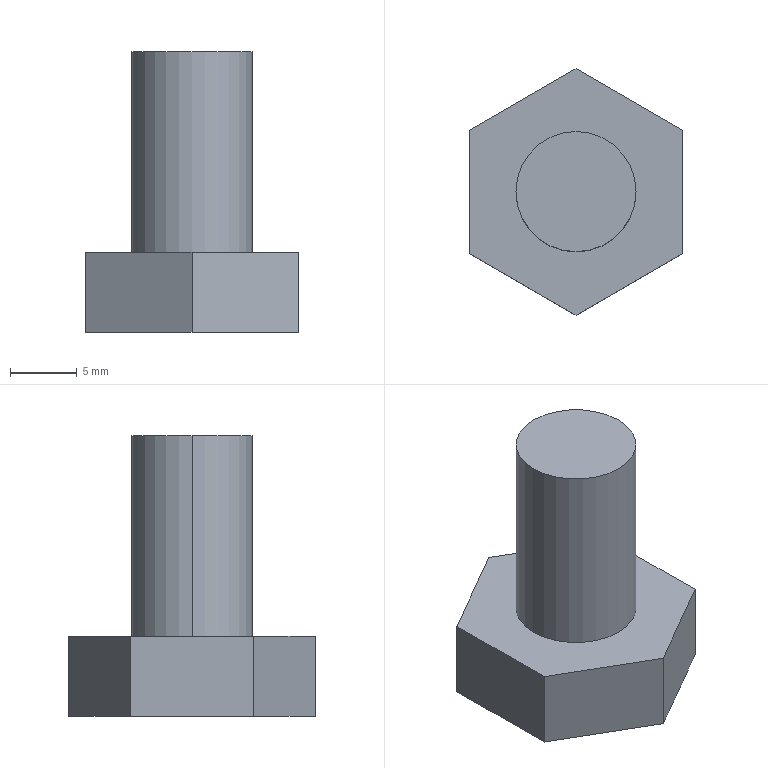Part | SolidWorks | features Extrusion 1, ICE 1 | 1 solid | 11 faces | box 16 x 18.475 x 21 mm | volume 2284 mm3 | plane 9 | cylinder 2 | commonest cylinder face diameters 9 x2
STEP:
#1=CARTESIAN_POINT('',(4.5,0.,21.));
#2=VERTEX_POINT('',#1);
#3=CARTESIAN_POINT('',(-4.5,0.,21.));
#4=VERTEX_POINT('',#3);
#5=CARTESIAN_POINT('',(0.,0.,21.));
#6=DIRECTION('',(0.,0.,1.));
#7=DIRECTION('',(1.,0.,0.));
#8=AXIS2_PLACEMENT_3D('',#5,#6,#7);
#9=CIRCLE('',#8,4.5);
#10=EDGE_CURVE('',#2,#4,#9,.T.);
#11=ORIENTED_EDGE('',*,*,#10,.F.);
#12=CARTESIAN_POINT('',(4.5,0.,6.));
#13=VERTEX_POINT('',#12);
#14=CARTESIAN_POINT('',(4.5,0.,21.));
#15=DIRECTION('',(0.,0.,-1.));
#16=VECTOR('',#15,1000.);
#17=LINE('',#14,#16);
#18=EDGE_CURVE('',#2,#13,#17,.T.);
#19=ORIENTED_EDGE('',*,*,#18,.T.);
#20=CARTESIAN_POINT('',(-4.5,0.,6.));
#21=VERTEX_POINT('',#20);
#22=CARTESIAN_POINT('',(0.,0.,6.));
#23=DIRECTION('',(0.,0.,1.));
#24=DIRECTION('',(1.,0.,0.));
#25=AXIS2_PLACEMENT_3D('',#22,#23,#24);
#26=CIRCLE('',#25,4.5);
#27=EDGE_CURVE('',#13,#21,#26,.T.);
#28=ORIENTED_EDGE('',*,*,#27,.T.);
#29=CARTESIAN_POINT('',(-4.5,0.,21.));
#30=DIRECTION('',(0.,0.,-1.));
#31=VECTOR('',#30,1000.);
#32=LINE('',#29,#31);
#33=EDGE_CURVE('',#4,#21,#32,.T.);
#34=ORIENTED_EDGE('',*,*,#33,.F.);
#35=EDGE_LOOP('',(#11,#19,#28,#34));
#36=FACE_OUTER_BOUND('',#35,.T.);
#37=CARTESIAN_POINT('',(0.,0.,21.));
#38=DIRECTION('',(0.,0.,-1.));
#39=DIRECTION('',(-1.,0.,0.));
#40=AXIS2_PLACEMENT_3D('',#37,#38,#39);
#41=CYLINDRICAL_SURFACE('',#40,4.5);
#42=ADVANCED_FACE('',(#36),#41,.T.);
#43=CARTESIAN_POINT('',(8.,4.619,0.));
#44=VERTEX_POINT('',#43);
#45=CARTESIAN_POINT('',(0.,9.238,0.));
#46=VERTEX_POINT('',#45);
#47=CARTESIAN_POINT('',(8.,4.619,0.));
#48=DIRECTION('',(-0.866,0.5,0.));
#49=VECTOR('',#48,1000.);
#50=LINE('',#47,#49);
#51=EDGE_CURVE('',#44,#46,#50,.T.);
#52=ORIENTED_EDGE('',*,*,#51,.T.);
#53=CARTESIAN_POINT('',(0.,9.238,6.));
#54=VERTEX_POINT('',#53);
#55=CARTESIAN_POINT('',(0.,9.238,6.));
#56=DIRECTION('',(0.,0.,-1.));
#57=VECTOR('',#56,1000.);
#58=LINE('',#55,#57);
#59=EDGE_CURVE('',#54,#46,#58,.T.);
#60=ORIENTED_EDGE('',*,*,#59,.F.);
#61=CARTESIAN_POINT('',(8.,4.619,6.));
#62=VERTEX_POINT('',#61);
#63=CARTESIAN_POINT('',(8.,4.619,6.));
#64=DIRECTION('',(-0.866,0.5,0.));
#65=VECTOR('',#64,1000.);
#66=LINE('',#63,#65);
#67=EDGE_CURVE('',#62,#54,#66,.T.);
#68=ORIENTED_EDGE('',*,*,#67,.F.);
#69=CARTESIAN_POINT('',(8.,4.619,6.));
#70=DIRECTION('',(0.,0.,-1.));
#71=VECTOR('',#70,1000.);
#72=LINE('',#69,#71);
#73=EDGE_CURVE('',#62,#44,#72,.T.);
#74=ORIENTED_EDGE('',*,*,#73,.T.);
#75=EDGE_LOOP('',(#52,#60,#68,#74));
#76=FACE_OUTER_BOUND('',#75,.T.);
#77=CARTESIAN_POINT('',(8.,4.619,6.));
#78=DIRECTION('',(-0.5,-0.866,0.));
#79=DIRECTION('',(0.866,-0.5,0.));
#80=AXIS2_PLACEMENT_3D('',#77,#78,#79);
#81=PLANE('',#80);
#82=ADVANCED_FACE('',(#76),#81,.F.);
#83=CARTESIAN_POINT('',(-8.,4.619,0.));
#84=VERTEX_POINT('',#83);
#85=CARTESIAN_POINT('',(0.,9.238,0.));
#86=DIRECTION('',(-0.866,-0.5,0.));
#87=VECTOR('',#86,1000.);
#88=LINE('',#85,#87);
#89=EDGE_CURVE('',#46,#84,#88,.T.);
#90=ORIENTED_EDGE('',*,*,#89,.T.);
#91=CARTESIAN_POINT('',(-8.,4.619,6.));
#92=VERTEX_POINT('',#91);
#93=CARTESIAN_POINT('',(-8.,4.619,6.));
#94=DIRECTION('',(0.,0.,-1.));
#95=VECTOR('',#94,1000.);
#96=LINE('',#93,#95);
#97=EDGE_CURVE('',#92,#84,#96,.T.);
#98=ORIENTED_EDGE('',*,*,#97,.F.);
#99=CARTESIAN_POINT('',(0.,9.238,6.));
#100=DIRECTION('',(-0.866,-0.5,0.));
#101=VECTOR('',#100,1000.);
#102=LINE('',#99,#101);
#103=EDGE_CURVE('',#54,#92,#102,.T.);
#104=ORIENTED_EDGE('',*,*,#103,.F.);
#105=ORIENTED_EDGE('',*,*,#59,.T.);
#106=EDGE_LOOP('',(#90,#98,#104,#105));
#107=FACE_OUTER_BOUND('',#106,.T.);
#108=CARTESIAN_POINT('',(0.,9.238,6.));
#109=DIRECTION('',(0.5,-0.866,0.));
#110=DIRECTION('',(0.866,0.5,0.));
#111=AXIS2_PLACEMENT_3D('',#108,#109,#110);
#112=PLANE('',#111);
#113=ADVANCED_FACE('',(#107),#112,.F.);
#114=CARTESIAN_POINT('',(-8.,-4.619,0.));
#115=VERTEX_POINT('',#114);
#116=CARTESIAN_POINT('',(-8.,4.619,0.));
#117=DIRECTION('',(0.,-1.,0.));
#118=VECTOR('',#117,1000.);
#119=LINE('',#116,#118);
#120=EDGE_CURVE('',#84,#115,#119,.T.);
#121=ORIENTED_EDGE('',*,*,#120,.T.);
#122=CARTESIAN_POINT('',(-8.,-4.619,6.));
#123=VERTEX_POINT('',#122);
#124=CARTESIAN_POINT('',(-8.,-4.619,6.));
#125=DIRECTION('',(0.,0.,-1.));
#126=VECTOR('',#125,1000.);
#127=LINE('',#124,#126);
#128=EDGE_CURVE('',#123,#115,#127,.T.);
#129=ORIENTED_EDGE('',*,*,#128,.F.);
#130=CARTESIAN_POINT('',(-8.,4.619,6.));
#131=DIRECTION('',(0.,-1.,0.));
#132=VECTOR('',#131,1000.);
#133=LINE('',#130,#132);
#134=EDGE_CURVE('',#92,#123,#133,.T.);
#135=ORIENTED_EDGE('',*,*,#134,.F.);
#136=ORIENTED_EDGE('',*,*,#97,.T.);
#137=EDGE_LOOP('',(#121,#129,#135,#136));
#138=FACE_OUTER_BOUND('',#137,.T.);
#139=CARTESIAN_POINT('',(-8.,4.619,6.));
#140=DIRECTION('',(1.,0.,0.));
#141=DIRECTION('',(0.,1.,0.));
#142=AXIS2_PLACEMENT_3D('',#139,#140,#141);
#143=PLANE('',#142);
#144=ADVANCED_FACE('',(#138),#143,.F.);
#145=CARTESIAN_POINT('',(0.,-9.238,0.));
#146=VERTEX_POINT('',#145);
#147=CARTESIAN_POINT('',(-8.,-4.619,0.));
#148=DIRECTION('',(0.866,-0.5,0.));
#149=VECTOR('',#148,1000.);
#150=LINE('',#147,#149);
#151=EDGE_CURVE('',#115,#146,#150,.T.);
#152=ORIENTED_EDGE('',*,*,#151,.T.);
#153=CARTESIAN_POINT('',(0.,-9.238,6.));
#154=VERTEX_POINT('',#153);
#155=CARTESIAN_POINT('',(0.,-9.238,6.));
#156=DIRECTION('',(0.,0.,-1.));
#157=VECTOR('',#156,1000.);
#158=LINE('',#155,#157);
#159=EDGE_CURVE('',#154,#146,#158,.T.);
#160=ORIENTED_EDGE('',*,*,#159,.F.);
#161=CARTESIAN_POINT('',(-8.,-4.619,6.));
#162=DIRECTION('',(0.866,-0.5,0.));
#163=VECTOR('',#162,1000.);
#164=LINE('',#161,#163);
#165=EDGE_CURVE('',#123,#154,#164,.T.);
#166=ORIENTED_EDGE('',*,*,#165,.F.);
#167=ORIENTED_EDGE('',*,*,#128,.T.);
#168=EDGE_LOOP('',(#152,#160,#166,#167));
#169=FACE_OUTER_BOUND('',#168,.T.);
#170=CARTESIAN_POINT('',(-8.,-4.619,6.));
#171=DIRECTION('',(0.5,0.866,0.));
#172=DIRECTION('',(-0.866,0.5,0.));
#173=AXIS2_PLACEMENT_3D('',#170,#171,#172);
#174=PLANE('',#173);
#175=ADVANCED_FACE('',(#169),#174,.F.);
#176=CARTESIAN_POINT('',(8.,-4.619,0.));
#177=VERTEX_POINT('',#176);
#178=CARTESIAN_POINT('',(0.,-9.238,0.));
#179=DIRECTION('',(0.866,0.5,0.));
#180=VECTOR('',#179,1000.);
#181=LINE('',#178,#180);
#182=EDGE_CURVE('',#146,#177,#181,.T.);
#183=ORIENTED_EDGE('',*,*,#182,.T.);
#184=CARTESIAN_POINT('',(8.,-4.619,6.));
#185=VERTEX_POINT('',#184);
#186=CARTESIAN_POINT('',(8.,-4.619,6.));
#187=DIRECTION('',(0.,0.,-1.));
#188=VECTOR('',#187,1000.);
#189=LINE('',#186,#188);
#190=EDGE_CURVE('',#185,#177,#189,.T.);
#191=ORIENTED_EDGE('',*,*,#190,.F.);
#192=CARTESIAN_POINT('',(0.,-9.238,6.));
#193=DIRECTION('',(0.866,0.5,0.));
#194=VECTOR('',#193,1000.);
#195=LINE('',#192,#194);
#196=EDGE_CURVE('',#154,#185,#195,.T.);
#197=ORIENTED_EDGE('',*,*,#196,.F.);
#198=ORIENTED_EDGE('',*,*,#159,.T.);
#199=EDGE_LOOP('',(#183,#191,#197,#198));
#200=FACE_OUTER_BOUND('',#199,.T.);
#201=CARTESIAN_POINT('',(0.,-9.238,6.));
#202=DIRECTION('',(-0.5,0.866,0.));
#203=DIRECTION('',(-0.866,-0.5,0.));
#204=AXIS2_PLACEMENT_3D('',#201,#202,#203);
#205=PLANE('',#204);
#206=ADVANCED_FACE('',(#200),#205,.F.);
#207=CARTESIAN_POINT('',(8.,-4.619,0.));
#208=DIRECTION('',(0.,1.,0.));
#209=VECTOR('',#208,1000.);
#210=LINE('',#207,#209);
#211=EDGE_CURVE('',#177,#44,#210,.T.);
#212=ORIENTED_EDGE('',*,*,#211,.T.);
#213=ORIENTED_EDGE('',*,*,#73,.F.);
#214=CARTESIAN_POINT('',(8.,-4.619,6.));
#215=DIRECTION('',(0.,1.,0.));
#216=VECTOR('',#215,1000.);
#217=LINE('',#214,#216);
#218=EDGE_CURVE('',#185,#62,#217,.T.);
#219=ORIENTED_EDGE('',*,*,#218,.F.);
#220=ORIENTED_EDGE('',*,*,#190,.T.);
#221=EDGE_LOOP('',(#212,#213,#219,#220));
#222=FACE_OUTER_BOUND('',#221,.T.);
#223=CARTESIAN_POINT('',(8.,-4.619,6.));
#224=DIRECTION('',(-1.,0.,0.));
#225=DIRECTION('',(0.,-1.,0.));
#226=AXIS2_PLACEMENT_3D('',#223,#224,#225);
#227=PLANE('',#226);
#228=ADVANCED_FACE('',(#222),#227,.F.);
#229=CARTESIAN_POINT('',(0.,0.,6.));
#230=DIRECTION('',(0.,0.,1.));
#231=DIRECTION('',(1.,0.,0.));
#232=AXIS2_PLACEMENT_3D('',#229,#230,#231);
#233=CIRCLE('',#232,4.5);
#234=EDGE_CURVE('',#21,#13,#233,.T.);
#235=ORIENTED_EDGE('',*,*,#234,.F.);
#236=ORIENTED_EDGE('',*,*,#27,.F.);
#237=EDGE_LOOP('',(#235,#236));
#238=FACE_BOUND('',#237,.T.);
#239=ORIENTED_EDGE('',*,*,#67,.T.);
#240=ORIENTED_EDGE('',*,*,#103,.T.);
#241=ORIENTED_EDGE('',*,*,#134,.T.);
#242=ORIENTED_EDGE('',*,*,#165,.T.);
#243=ORIENTED_EDGE('',*,*,#196,.T.);
#244=ORIENTED_EDGE('',*,*,#218,.T.);
#245=EDGE_LOOP('',(#239,#240,#241,#242,#243,#244));
#246=FACE_OUTER_BOUND('',#245,.T.);
#247=CARTESIAN_POINT('',(0.,0.,6.));
#248=DIRECTION('',(0.,0.,1.));
#249=DIRECTION('',(1.,0.,0.));
#250=AXIS2_PLACEMENT_3D('',#247,#248,#249);
#251=PLANE('',#250);
#252=ADVANCED_FACE('',(#238,#246),#251,.T.);
#253=ORIENTED_EDGE('',*,*,#51,.F.);
#254=ORIENTED_EDGE('',*,*,#211,.F.);
#255=ORIENTED_EDGE('',*,*,#182,.F.);
#256=ORIENTED_EDGE('',*,*,#151,.F.);
#257=ORIENTED_EDGE('',*,*,#120,.F.);
#258=ORIENTED_EDGE('',*,*,#89,.F.);
#259=EDGE_LOOP('',(#253,#254,#255,#256,#257,#258));
#260=FACE_OUTER_BOUND('',#259,.T.);
#261=CARTESIAN_POINT('',(0.,0.,0.));
#262=DIRECTION('',(0.,0.,1.));
#263=DIRECTION('',(1.,0.,0.));
#264=AXIS2_PLACEMENT_3D('',#261,#262,#263);
#265=PLANE('',#264);
#266=ADVANCED_FACE('',(#260),#265,.F.);
#267=ORIENTED_EDGE('',*,*,#18,.F.);
#268=CARTESIAN_POINT('',(0.,0.,21.));
#269=DIRECTION('',(0.,0.,1.));
#270=DIRECTION('',(1.,0.,0.));
#271=AXIS2_PLACEMENT_3D('',#268,#269,#270);
#272=CIRCLE('',#271,4.5);
#273=EDGE_CURVE('',#4,#2,#272,.T.);
#274=ORIENTED_EDGE('',*,*,#273,.F.);
#275=ORIENTED_EDGE('',*,*,#33,.T.);
#276=ORIENTED_EDGE('',*,*,#234,.T.);
#277=EDGE_LOOP('',(#267,#274,#275,#276));
#278=FACE_OUTER_BOUND('',#277,.T.);
#279=CARTESIAN_POINT('',(0.,0.,21.));
#280=DIRECTION('',(0.,0.,-1.));
#281=DIRECTION('',(-1.,0.,0.));
#282=AXIS2_PLACEMENT_3D('',#279,#280,#281);
#283=CYLINDRICAL_SURFACE('',#282,4.5);
#284=ADVANCED_FACE('',(#278),#283,.T.);
#285=ORIENTED_EDGE('',*,*,#273,.T.);
#286=ORIENTED_EDGE('',*,*,#10,.T.);
#287=EDGE_LOOP('',(#285,#286));
#288=FACE_OUTER_BOUND('',#287,.T.);
#289=CARTESIAN_POINT('',(0.,0.,21.));
#290=DIRECTION('',(0.,0.,1.));
#291=DIRECTION('',(1.,0.,0.));
#292=AXIS2_PLACEMENT_3D('',#289,#290,#291);
#293=PLANE('',#292);
#294=ADVANCED_FACE('',(#288),#293,.T.);
#295=CLOSED_SHELL('',(#42,#82,#113,#144,#175,#206,#228,#252,#266,#284,#294));
#296=MANIFOLD_SOLID_BREP('',#295);
#297=CARTESIAN_POINT('',(0.,0.,0.));
#298=DIRECTION('',(0.,0.,1.));
#299=DIRECTION('',(1.,0.,0.));
#300=AXIS2_PLACEMENT_3D('',#297,#298,#299);
#301=(LENGTH_UNIT()NAMED_UNIT(*)SI_UNIT(.MILLI.,.METRE.));
#302=UNCERTAINTY_MEASURE_WITH_UNIT(LENGTH_MEASURE(0.00001),#301,'','');
#303=(NAMED_UNIT(*)PLANE_ANGLE_UNIT()SI_UNIT($,.RADIAN.));
#304=(NAMED_UNIT(*)SI_UNIT($,.STERADIAN.)SOLID_ANGLE_UNIT());
#305=(GEOMETRIC_REPRESENTATION_CONTEXT(3)GLOBAL_UNCERTAINTY_ASSIGNED_CONTEXT((#302))GLOBAL_UNIT_ASSIGNED_CONTEXT((#301,#303,#304))REPRESENTATION_CONTEXT('',''));
#306=ADVANCED_BREP_SHAPE_REPRESENTATION('',(#296,#300),#305);